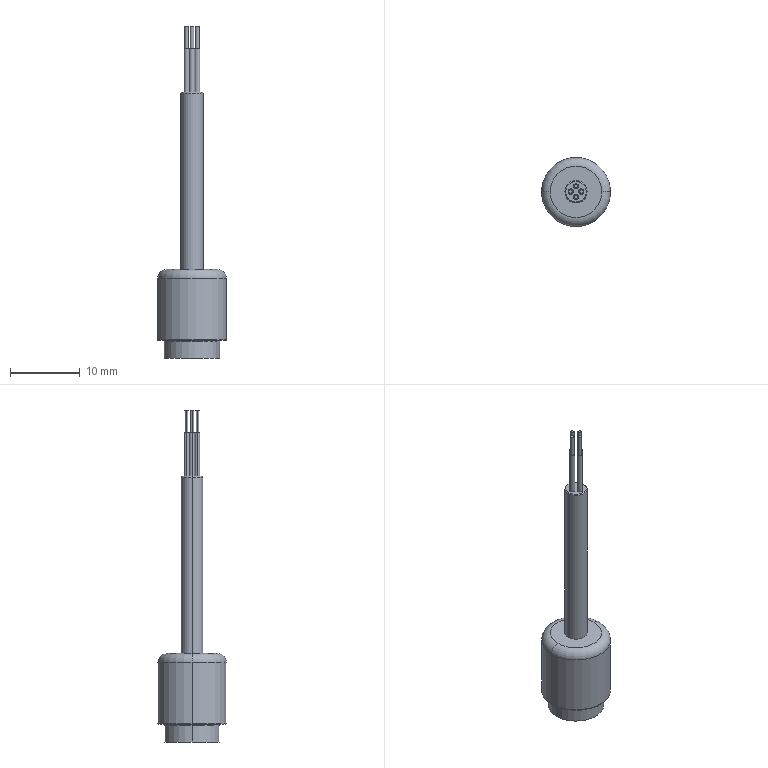Part | STEP file | CABLE | 1 solid | 42 faces | box 9.906 x 9.906 x 47.625 mm | volume 1114 mm3 | cylinder 22 | plane 12 | torus 8 | commonest cylinder face diameters 0.508 x8 0.762 x8 3.175 x2 7.938 x2 9.906 x2
STEP:
#1=CARTESIAN_POINT('',(-1.587,0.,35.433));
#2=VERTEX_POINT('',#1);
#3=CARTESIAN_POINT('',(1.587,0.,35.433));
#4=VERTEX_POINT('',#3);
#5=CARTESIAN_POINT('',(0.,0.,35.433));
#6=DIRECTION('',(0.,0.,-1.));
#7=DIRECTION('',(1.,0.,0.));
#8=AXIS2_PLACEMENT_3D('',#5,#6,#7);
#9=CIRCLE('',#8,1.587);
#10=EDGE_CURVE('',#2,#4,#9,.T.);
#11=ORIENTED_EDGE('',*,*,#10,.F.);
#12=CARTESIAN_POINT('',(-1.46,0.,35.56));
#13=VERTEX_POINT('',#12);
#14=CARTESIAN_POINT('',(-1.46,0.,35.433));
#15=DIRECTION('',(0.,1.,0.));
#16=DIRECTION('',(-1.,0.,0.));
#17=AXIS2_PLACEMENT_3D('',#14,#15,#16);
#18=CIRCLE('',#17,0.127);
#19=EDGE_CURVE('',#2,#13,#18,.T.);
#20=ORIENTED_EDGE('',*,*,#19,.T.);
#21=CARTESIAN_POINT('',(1.46,0.,35.56));
#22=VERTEX_POINT('',#21);
#23=CARTESIAN_POINT('',(0.,0.,35.56));
#24=DIRECTION('',(0.,0.,1.));
#25=DIRECTION('',(1.,0.,0.));
#26=AXIS2_PLACEMENT_3D('',#23,#24,#25);
#27=CIRCLE('',#26,1.46);
#28=EDGE_CURVE('',#22,#13,#27,.T.);
#29=ORIENTED_EDGE('',*,*,#28,.F.);
#30=CARTESIAN_POINT('',(1.46,0.,35.433));
#31=DIRECTION('',(0.,-1.,0.));
#32=DIRECTION('',(0.,0.,-1.));
#33=AXIS2_PLACEMENT_3D('',#30,#31,#32);
#34=CIRCLE('',#33,0.127);
#35=EDGE_CURVE('',#4,#22,#34,.T.);
#36=ORIENTED_EDGE('',*,*,#35,.F.);
#37=EDGE_LOOP('',(#11,#20,#29,#36));
#38=FACE_OUTER_BOUND('',#37,.T.);
#39=CARTESIAN_POINT('',(0.,0.,35.433));
#40=DIRECTION('',(0.,0.,1.));
#41=DIRECTION('',(1.,0.,0.));
#42=AXIS2_PLACEMENT_3D('',#39,#40,#41);
#43=TOROIDAL_SURFACE('',#42,1.46,0.127);
#44=ADVANCED_FACE('',(#38),#43,.T.);
#45=CARTESIAN_POINT('',(-0.508,0.,45.085));
#46=VERTEX_POINT('',#45);
#47=CARTESIAN_POINT('',(-1.016,0.,45.085));
#48=VERTEX_POINT('',#47);
#49=CARTESIAN_POINT('',(-0.762,0.,45.085));
#50=DIRECTION('',(0.,0.,1.));
#51=DIRECTION('',(1.,0.,0.));
#52=AXIS2_PLACEMENT_3D('',#49,#50,#51);
#53=CIRCLE('',#52,0.254);
#54=EDGE_CURVE('',#46,#48,#53,.T.);
#55=ORIENTED_EDGE('',*,*,#54,.F.);
#56=CARTESIAN_POINT('',(-0.508,0.,41.91));
#57=VERTEX_POINT('',#56);
#58=CARTESIAN_POINT('',(-0.508,0.,45.085));
#59=DIRECTION('',(0.,0.,-1.));
#60=VECTOR('',#59,1000.);
#61=LINE('',#58,#60);
#62=EDGE_CURVE('',#46,#57,#61,.T.);
#63=ORIENTED_EDGE('',*,*,#62,.T.);
#64=CARTESIAN_POINT('',(-1.016,0.,41.91));
#65=VERTEX_POINT('',#64);
#66=CARTESIAN_POINT('',(-0.762,0.,41.91));
#67=DIRECTION('',(0.,0.,-1.));
#68=DIRECTION('',(1.,0.,0.));
#69=AXIS2_PLACEMENT_3D('',#66,#67,#68);
#70=CIRCLE('',#69,0.254);
#71=EDGE_CURVE('',#65,#57,#70,.T.);
#72=ORIENTED_EDGE('',*,*,#71,.F.);
#73=CARTESIAN_POINT('',(-1.016,0.,45.085));
#74=DIRECTION('',(0.,0.,-1.));
#75=VECTOR('',#74,1000.);
#76=LINE('',#73,#75);
#77=EDGE_CURVE('',#48,#65,#76,.T.);
#78=ORIENTED_EDGE('',*,*,#77,.F.);
#79=EDGE_LOOP('',(#55,#63,#72,#78));
#80=FACE_OUTER_BOUND('',#79,.T.);
#81=CARTESIAN_POINT('',(-0.762,0.,45.085));
#82=DIRECTION('',(0.,0.,-1.));
#83=DIRECTION('',(-1.,0.,0.));
#84=AXIS2_PLACEMENT_3D('',#81,#82,#83);
#85=CYLINDRICAL_SURFACE('',#84,0.254);
#86=ADVANCED_FACE('',(#80),#85,.T.);
#87=CARTESIAN_POINT('',(-0.381,0.,41.91));
#88=VERTEX_POINT('',#87);
#89=CARTESIAN_POINT('',(-1.143,0.,41.91));
#90=VERTEX_POINT('',#89);
#91=CARTESIAN_POINT('',(-0.762,0.,41.91));
#92=DIRECTION('',(0.,0.,1.));
#93=DIRECTION('',(1.,0.,0.));
#94=AXIS2_PLACEMENT_3D('',#91,#92,#93);
#95=CIRCLE('',#94,0.381);
#96=EDGE_CURVE('',#88,#90,#95,.T.);
#97=ORIENTED_EDGE('',*,*,#96,.F.);
#98=CARTESIAN_POINT('',(-0.381,0.,35.56));
#99=VERTEX_POINT('',#98);
#100=CARTESIAN_POINT('',(-0.381,0.,41.91));
#101=DIRECTION('',(0.,0.,-1.));
#102=VECTOR('',#101,1000.);
#103=LINE('',#100,#102);
#104=EDGE_CURVE('',#88,#99,#103,.T.);
#105=ORIENTED_EDGE('',*,*,#104,.T.);
#106=CARTESIAN_POINT('',(-1.143,0.,35.56));
#107=VERTEX_POINT('',#106);
#108=CARTESIAN_POINT('',(-0.762,0.,35.56));
#109=DIRECTION('',(0.,0.,1.));
#110=DIRECTION('',(1.,0.,0.));
#111=AXIS2_PLACEMENT_3D('',#108,#109,#110);
#112=CIRCLE('',#111,0.381);
#113=EDGE_CURVE('',#99,#107,#112,.T.);
#114=ORIENTED_EDGE('',*,*,#113,.T.);
#115=CARTESIAN_POINT('',(-1.143,0.,41.91));
#116=DIRECTION('',(0.,0.,-1.));
#117=VECTOR('',#116,1000.);
#118=LINE('',#115,#117);
#119=EDGE_CURVE('',#90,#107,#118,.T.);
#120=ORIENTED_EDGE('',*,*,#119,.F.);
#121=EDGE_LOOP('',(#97,#105,#114,#120));
#122=FACE_OUTER_BOUND('',#121,.T.);
#123=CARTESIAN_POINT('',(-0.762,0.,41.91));
#124=DIRECTION('',(0.,0.,-1.));
#125=DIRECTION('',(-1.,0.,0.));
#126=AXIS2_PLACEMENT_3D('',#123,#124,#125);
#127=CYLINDRICAL_SURFACE('',#126,0.381);
#128=ADVANCED_FACE('',(#122),#127,.T.);
#129=CARTESIAN_POINT('',(0.254,0.762,45.085));
#130=VERTEX_POINT('',#129);
#131=CARTESIAN_POINT('',(-0.254,0.762,45.085));
#132=VERTEX_POINT('',#131);
#133=CARTESIAN_POINT('',(0.,0.762,45.085));
#134=DIRECTION('',(0.,0.,1.));
#135=DIRECTION('',(1.,0.,0.));
#136=AXIS2_PLACEMENT_3D('',#133,#134,#135);
#137=CIRCLE('',#136,0.254);
#138=EDGE_CURVE('',#130,#132,#137,.T.);
#139=ORIENTED_EDGE('',*,*,#138,.F.);
#140=CARTESIAN_POINT('',(0.254,0.762,41.91));
#141=VERTEX_POINT('',#140);
#142=CARTESIAN_POINT('',(0.254,0.762,45.085));
#143=DIRECTION('',(0.,0.,-1.));
#144=VECTOR('',#143,1000.);
#145=LINE('',#142,#144);
#146=EDGE_CURVE('',#130,#141,#145,.T.);
#147=ORIENTED_EDGE('',*,*,#146,.T.);
#148=CARTESIAN_POINT('',(-0.254,0.762,41.91));
#149=VERTEX_POINT('',#148);
#150=CARTESIAN_POINT('',(0.,0.762,41.91));
#151=DIRECTION('',(0.,0.,-1.));
#152=DIRECTION('',(1.,0.,0.));
#153=AXIS2_PLACEMENT_3D('',#150,#151,#152);
#154=CIRCLE('',#153,0.254);
#155=EDGE_CURVE('',#149,#141,#154,.T.);
#156=ORIENTED_EDGE('',*,*,#155,.F.);
#157=CARTESIAN_POINT('',(-0.254,0.762,45.085));
#158=DIRECTION('',(0.,0.,-1.));
#159=VECTOR('',#158,1000.);
#160=LINE('',#157,#159);
#161=EDGE_CURVE('',#132,#149,#160,.T.);
#162=ORIENTED_EDGE('',*,*,#161,.F.);
#163=EDGE_LOOP('',(#139,#147,#156,#162));
#164=FACE_OUTER_BOUND('',#163,.T.);
#165=CARTESIAN_POINT('',(0.,0.762,45.085));
#166=DIRECTION('',(0.,0.,-1.));
#167=DIRECTION('',(-1.,0.,0.));
#168=AXIS2_PLACEMENT_3D('',#165,#166,#167);
#169=CYLINDRICAL_SURFACE('',#168,0.254);
#170=ADVANCED_FACE('',(#164),#169,.T.);
#171=CARTESIAN_POINT('',(0.381,0.762,41.91));
#172=VERTEX_POINT('',#171);
#173=CARTESIAN_POINT('',(-0.381,0.762,41.91));
#174=VERTEX_POINT('',#173);
#175=CARTESIAN_POINT('',(0.,0.762,41.91));
#176=DIRECTION('',(0.,0.,1.));
#177=DIRECTION('',(1.,0.,0.));
#178=AXIS2_PLACEMENT_3D('',#175,#176,#177);
#179=CIRCLE('',#178,0.381);
#180=EDGE_CURVE('',#172,#174,#179,.T.);
#181=ORIENTED_EDGE('',*,*,#180,.F.);
#182=CARTESIAN_POINT('',(0.381,0.762,35.56));
#183=VERTEX_POINT('',#182);
#184=CARTESIAN_POINT('',(0.381,0.762,41.91));
#185=DIRECTION('',(0.,0.,-1.));
#186=VECTOR('',#185,1000.);
#187=LINE('',#184,#186);
#188=EDGE_CURVE('',#172,#183,#187,.T.);
#189=ORIENTED_EDGE('',*,*,#188,.T.);
#190=CARTESIAN_POINT('',(-0.381,0.762,35.56));
#191=VERTEX_POINT('',#190);
#192=CARTESIAN_POINT('',(0.,0.762,35.56));
#193=DIRECTION('',(0.,0.,1.));
#194=DIRECTION('',(1.,0.,0.));
#195=AXIS2_PLACEMENT_3D('',#192,#193,#194);
#196=CIRCLE('',#195,0.381);
#197=EDGE_CURVE('',#183,#191,#196,.T.);
#198=ORIENTED_EDGE('',*,*,#197,.T.);
#199=CARTESIAN_POINT('',(-0.381,0.762,41.91));
#200=DIRECTION('',(0.,0.,-1.));
#201=VECTOR('',#200,1000.);
#202=LINE('',#199,#201);
#203=EDGE_CURVE('',#174,#191,#202,.T.);
#204=ORIENTED_EDGE('',*,*,#203,.F.);
#205=EDGE_LOOP('',(#181,#189,#198,#204));
#206=FACE_OUTER_BOUND('',#205,.T.);
#207=CARTESIAN_POINT('',(0.,0.762,41.91));
#208=DIRECTION('',(0.,0.,-1.));
#209=DIRECTION('',(-1.,0.,0.));
#210=AXIS2_PLACEMENT_3D('',#207,#208,#209);
#211=CYLINDRICAL_SURFACE('',#210,0.381);
#212=ADVANCED_FACE('',(#206),#211,.T.);
#213=CARTESIAN_POINT('',(1.016,0.,45.085));
#214=VERTEX_POINT('',#213);
#215=CARTESIAN_POINT('',(0.508,0.,45.085));
#216=VERTEX_POINT('',#215);
#217=CARTESIAN_POINT('',(0.762,0.,45.085));
#218=DIRECTION('',(0.,0.,1.));
#219=DIRECTION('',(1.,0.,0.));
#220=AXIS2_PLACEMENT_3D('',#217,#218,#219);
#221=CIRCLE('',#220,0.254);
#222=EDGE_CURVE('',#214,#216,#221,.T.);
#223=ORIENTED_EDGE('',*,*,#222,.F.);
#224=CARTESIAN_POINT('',(1.016,0.,41.91));
#225=VERTEX_POINT('',#224);
#226=CARTESIAN_POINT('',(1.016,0.,45.085));
#227=DIRECTION('',(0.,0.,-1.));
#228=VECTOR('',#227,1000.);
#229=LINE('',#226,#228);
#230=EDGE_CURVE('',#214,#225,#229,.T.);
#231=ORIENTED_EDGE('',*,*,#230,.T.);
#232=CARTESIAN_POINT('',(0.508,0.,41.91));
#233=VERTEX_POINT('',#232);
#234=CARTESIAN_POINT('',(0.762,0.,41.91));
#235=DIRECTION('',(0.,0.,-1.));
#236=DIRECTION('',(1.,0.,0.));
#237=AXIS2_PLACEMENT_3D('',#234,#235,#236);
#238=CIRCLE('',#237,0.254);
#239=EDGE_CURVE('',#233,#225,#238,.T.);
#240=ORIENTED_EDGE('',*,*,#239,.F.);
#241=CARTESIAN_POINT('',(0.508,0.,45.085));
#242=DIRECTION('',(0.,0.,-1.));
#243=VECTOR('',#242,1000.);
#244=LINE('',#241,#243);
#245=EDGE_CURVE('',#216,#233,#244,.T.);
#246=ORIENTED_EDGE('',*,*,#245,.F.);
#247=EDGE_LOOP('',(#223,#231,#240,#246));
#248=FACE_OUTER_BOUND('',#247,.T.);
#249=CARTESIAN_POINT('',(0.762,0.,45.085));
#250=DIRECTION('',(0.,0.,-1.));
#251=DIRECTION('',(-1.,0.,0.));
#252=AXIS2_PLACEMENT_3D('',#249,#250,#251);
#253=CYLINDRICAL_SURFACE('',#252,0.254);
#254=ADVANCED_FACE('',(#248),#253,.T.);
#255=CARTESIAN_POINT('',(1.143,0.,41.91));
#256=VERTEX_POINT('',#255);
#257=CARTESIAN_POINT('',(0.381,0.,41.91));
#258=VERTEX_POINT('',#257);
#259=CARTESIAN_POINT('',(0.762,0.,41.91));
#260=DIRECTION('',(0.,0.,1.));
#261=DIRECTION('',(1.,0.,0.));
#262=AXIS2_PLACEMENT_3D('',#259,#260,#261);
#263=CIRCLE('',#262,0.381);
#264=EDGE_CURVE('',#256,#258,#263,.T.);
#265=ORIENTED_EDGE('',*,*,#264,.F.);
#266=CARTESIAN_POINT('',(1.143,0.,35.56));
#267=VERTEX_POINT('',#266);
#268=CARTESIAN_POINT('',(1.143,0.,41.91));
#269=DIRECTION('',(0.,0.,-1.));
#270=VECTOR('',#269,1000.);
#271=LINE('',#268,#270);
#272=EDGE_CURVE('',#256,#267,#271,.T.);
#273=ORIENTED_EDGE('',*,*,#272,.T.);
#274=CARTESIAN_POINT('',(0.381,0.,35.56));
#275=VERTEX_POINT('',#274);
#276=CARTESIAN_POINT('',(0.762,0.,35.56));
#277=DIRECTION('',(0.,0.,1.));
#278=DIRECTION('',(1.,0.,0.));
#279=AXIS2_PLACEMENT_3D('',#276,#277,#278);
#280=CIRCLE('',#279,0.381);
#281=EDGE_CURVE('',#267,#275,#280,.T.);
#282=ORIENTED_EDGE('',*,*,#281,.T.);
#283=CARTESIAN_POINT('',(0.381,0.,41.91));
#284=DIRECTION('',(0.,0.,-1.));
#285=VECTOR('',#284,1000.);
#286=LINE('',#283,#285);
#287=EDGE_CURVE('',#258,#275,#286,.T.);
#288=ORIENTED_EDGE('',*,*,#287,.F.);
#289=EDGE_LOOP('',(#265,#273,#282,#288));
#290=FACE_OUTER_BOUND('',#289,.T.);
#291=CARTESIAN_POINT('',(0.762,0.,41.91));
#292=DIRECTION('',(0.,0.,-1.));
#293=DIRECTION('',(-1.,0.,0.));
#294=AXIS2_PLACEMENT_3D('',#291,#292,#293);
#295=CYLINDRICAL_SURFACE('',#294,0.381);
#296=ADVANCED_FACE('',(#290),#295,.T.);
#297=CARTESIAN_POINT('',(0.254,-0.762,45.085));
#298=VERTEX_POINT('',#297);
#299=CARTESIAN_POINT('',(-0.254,-0.762,45.085));
#300=VERTEX_POINT('',#299);
#301=CARTESIAN_POINT('',(0.,-0.762,45.085));
#302=DIRECTION('',(0.,0.,1.));
#303=DIRECTION('',(1.,0.,0.));
#304=AXIS2_PLACEMENT_3D('',#301,#302,#303);
#305=CIRCLE('',#304,0.254);
#306=EDGE_CURVE('',#298,#300,#305,.T.);
#307=ORIENTED_EDGE('',*,*,#306,.F.);
#308=CARTESIAN_POINT('',(0.254,-0.762,41.91));
#309=VERTEX_POINT('',#308);
#310=CARTESIAN_POINT('',(0.254,-0.762,45.085));
#311=DIRECTION('',(0.,0.,-1.));
#312=VECTOR('',#311,1000.);
#313=LINE('',#310,#312);
#314=EDGE_CURVE('',#298,#309,#313,.T.);
#315=ORIENTED_EDGE('',*,*,#314,.T.);
#316=CARTESIAN_POINT('',(-0.254,-0.762,41.91));
#317=VERTEX_POINT('',#316);
#318=CARTESIAN_POINT('',(0.,-0.762,41.91));
#319=DIRECTION('',(0.,0.,-1.));
#320=DIRECTION('',(1.,0.,0.));
#321=AXIS2_PLACEMENT_3D('',#318,#319,#320);
#322=CIRCLE('',#321,0.254);
#323=EDGE_CURVE('',#317,#309,#322,.T.);
#324=ORIENTED_EDGE('',*,*,#323,.F.);
#325=CARTESIAN_POINT('',(-0.254,-0.762,45.085));
#326=DIRECTION('',(0.,0.,-1.));
#327=VECTOR('',#326,1000.);
#328=LINE('',#325,#327);
#329=EDGE_CURVE('',#300,#317,#328,.T.);
#330=ORIENTED_EDGE('',*,*,#329,.F.);
#331=EDGE_LOOP('',(#307,#315,#324,#330));
#332=FACE_OUTER_BOUND('',#331,.T.);
#333=CARTESIAN_POINT('',(0.,-0.762,45.085));
#334=DIRECTION('',(0.,0.,-1.));
#335=DIRECTION('',(-1.,0.,0.));
#336=AXIS2_PLACEMENT_3D('',#333,#334,#335);
#337=CYLINDRICAL_SURFACE('',#336,0.254);
#338=ADVANCED_FACE('',(#332),#337,.T.);
#339=CARTESIAN_POINT('',(0.381,-0.762,41.91));
#340=VERTEX_POINT('',#339);
#341=CARTESIAN_POINT('',(-0.381,-0.762,41.91));
#342=VERTEX_POINT('',#341);
#343=CARTESIAN_POINT('',(0.,-0.762,41.91));
#344=DIRECTION('',(0.,0.,1.));
#345=DIRECTION('',(1.,0.,0.));
#346=AXIS2_PLACEMENT_3D('',#343,#344,#345);
#347=CIRCLE('',#346,0.381);
#348=EDGE_CURVE('',#340,#342,#347,.T.);
#349=ORIENTED_EDGE('',*,*,#348,.F.);
#350=CARTESIAN_POINT('',(0.381,-0.762,35.56));
#351=VERTEX_POINT('',#350);
#352=CARTESIAN_POINT('',(0.381,-0.762,41.91));
#353=DIRECTION('',(0.,0.,-1.));
#354=VECTOR('',#353,1000.);
#355=LINE('',#352,#354);
#356=EDGE_CURVE('',#340,#351,#355,.T.);
#357=ORIENTED_EDGE('',*,*,#356,.T.);
#358=CARTESIAN_POINT('',(-0.381,-0.762,35.56));
#359=VERTEX_POINT('',#358);
#360=CARTESIAN_POINT('',(0.,-0.762,35.56));
#361=DIRECTION('',(0.,0.,1.));
#362=DIRECTION('',(1.,0.,0.));
#363=AXIS2_PLACEMENT_3D('',#360,#361,#362);
#364=CIRCLE('',#363,0.381);
#365=EDGE_CURVE('',#351,#359,#364,.T.);
#366=ORIENTED_EDGE('',*,*,#365,.T.);
#367=CARTESIAN_POINT('',(-0.381,-0.762,41.91));
#368=DIRECTION('',(0.,0.,-1.));
#369=VECTOR('',#368,1000.);
#370=LINE('',#367,#369);
#371=EDGE_CURVE('',#342,#359,#370,.T.);
#372=ORIENTED_EDGE('',*,*,#371,.F.);
#373=EDGE_LOOP('',(#349,#357,#366,#372));
#374=FACE_OUTER_BOUND('',#373,.T.);
#375=CARTESIAN_POINT('',(0.,-0.762,41.91));
#376=DIRECTION('',(0.,0.,-1.));
#377=DIRECTION('',(-1.,0.,0.));
#378=AXIS2_PLACEMENT_3D('',#375,#376,#377);
#379=CYLINDRICAL_SURFACE('',#378,0.381);
#380=ADVANCED_FACE('',(#374),#379,.T.);
#381=CARTESIAN_POINT('',(-4.953,0.,8.89));
#382=VERTEX_POINT('',#381);
#383=CARTESIAN_POINT('',(4.953,0.,8.89));
#384=VERTEX_POINT('',#383);
#385=CARTESIAN_POINT('',(0.,0.,8.89));
#386=DIRECTION('',(0.,0.,-1.));
#387=DIRECTION('',(1.,0.,0.));
#388=AXIS2_PLACEMENT_3D('',#385,#386,#387);
#389=CIRCLE('',#388,4.953);
#390=EDGE_CURVE('',#382,#384,#389,.T.);
#391=ORIENTED_EDGE('',*,*,#390,.F.);
#392=CARTESIAN_POINT('',(-3.683,0.,10.16));
#393=VERTEX_POINT('',#392);
#394=CARTESIAN_POINT('',(-3.683,0.,8.89));
#395=DIRECTION('',(0.,1.,0.));
#396=DIRECTION('',(-1.,0.,0.));
#397=AXIS2_PLACEMENT_3D('',#394,#395,#396);
#398=CIRCLE('',#397,1.27);
#399=EDGE_CURVE('',#382,#393,#398,.T.);
#400=ORIENTED_EDGE('',*,*,#399,.T.);
#401=CARTESIAN_POINT('',(3.683,0.,10.16));
#402=VERTEX_POINT('',#401);
#403=CARTESIAN_POINT('',(0.,0.,10.16));
#404=DIRECTION('',(0.,0.,1.));
#405=DIRECTION('',(1.,0.,0.));
#406=AXIS2_PLACEMENT_3D('',#403,#404,#405);
#407=CIRCLE('',#406,3.683);
#408=EDGE_CURVE('',#402,#393,#407,.T.);
#409=ORIENTED_EDGE('',*,*,#408,.F.);
#410=CARTESIAN_POINT('',(3.683,0.,8.89));
#411=DIRECTION('',(0.,-1.,0.));
#412=DIRECTION('',(0.,0.,-1.));
#413=AXIS2_PLACEMENT_3D('',#410,#411,#412);
#414=CIRCLE('',#413,1.27);
#415=EDGE_CURVE('',#384,#402,#414,.T.);
#416=ORIENTED_EDGE('',*,*,#415,.F.);
#417=EDGE_LOOP('',(#391,#400,#409,#416));
#418=FACE_OUTER_BOUND('',#417,.T.);
#419=CARTESIAN_POINT('',(0.,0.,8.89));
#420=DIRECTION('',(0.,0.,1.));
#421=DIRECTION('',(1.,0.,0.));
#422=AXIS2_PLACEMENT_3D('',#419,#420,#421);
#423=TOROIDAL_SURFACE('',#422,3.683,1.27);
#424=ADVANCED_FACE('',(#418),#423,.T.);
#425=CARTESIAN_POINT('',(-4.826,0.,0.));
#426=VERTEX_POINT('',#425);
#427=CARTESIAN_POINT('',(4.826,0.,0.));
#428=VERTEX_POINT('',#427);
#429=CARTESIAN_POINT('',(0.,0.,0.));
#430=DIRECTION('',(0.,0.,-1.));
#431=DIRECTION('',(1.,0.,0.));
#432=AXIS2_PLACEMENT_3D('',#429,#430,#431);
#433=CIRCLE('',#432,4.826);
#434=EDGE_CURVE('',#426,#428,#433,.T.);
#435=ORIENTED_EDGE('',*,*,#434,.F.);
#436=CARTESIAN_POINT('',(-4.953,0.,0.127));
#437=VERTEX_POINT('',#436);
#438=CARTESIAN_POINT('',(-4.826,0.,0.127));
#439=DIRECTION('',(0.,1.,0.));
#440=DIRECTION('',(-1.,0.,0.));
#441=AXIS2_PLACEMENT_3D('',#438,#439,#440);
#442=CIRCLE('',#441,0.127);
#443=EDGE_CURVE('',#426,#437,#442,.T.);
#444=ORIENTED_EDGE('',*,*,#443,.T.);
#445=CARTESIAN_POINT('',(4.953,0.,0.127));
#446=VERTEX_POINT('',#445);
#447=CARTESIAN_POINT('',(0.,0.,0.127));
#448=DIRECTION('',(0.,0.,1.));
#449=DIRECTION('',(1.,0.,0.));
#450=AXIS2_PLACEMENT_3D('',#447,#448,#449);
#451=CIRCLE('',#450,4.953);
#452=EDGE_CURVE('',#446,#437,#451,.T.);
#453=ORIENTED_EDGE('',*,*,#452,.F.);
#454=CARTESIAN_POINT('',(4.826,0.,0.127));
#455=DIRECTION('',(0.,-1.,0.));
#456=DIRECTION('',(0.,0.,-1.));
#457=AXIS2_PLACEMENT_3D('',#454,#455,#456);
#458=CIRCLE('',#457,0.127);
#459=EDGE_CURVE('',#428,#446,#458,.T.);
#460=ORIENTED_EDGE('',*,*,#459,.F.);
#461=EDGE_LOOP('',(#435,#444,#453,#460));
#462=FACE_OUTER_BOUND('',#461,.T.);
#463=CARTESIAN_POINT('',(0.,0.,0.127));
#464=DIRECTION('',(0.,0.,1.));
#465=DIRECTION('',(1.,0.,0.));
#466=AXIS2_PLACEMENT_3D('',#463,#464,#465);
#467=TOROIDAL_SURFACE('',#466,4.826,0.127);
#468=ADVANCED_FACE('',(#462),#467,.T.);
#469=CARTESIAN_POINT('',(-4.096,0.,0.));
#470=VERTEX_POINT('',#469);
#471=CARTESIAN_POINT('',(4.096,0.,0.));
#472=VERTEX_POINT('',#471);
#473=CARTESIAN_POINT('',(0.,0.,0.));
#474=DIRECTION('',(0.,0.,1.));
#475=DIRECTION('',(1.,0.,0.));
#476=AXIS2_PLACEMENT_3D('',#473,#474,#475);
#477=CIRCLE('',#476,4.096);
#478=EDGE_CURVE('',#470,#472,#477,.T.);
#479=ORIENTED_EDGE('',*,*,#478,.F.);
#480=CARTESIAN_POINT('',(-3.969,0.,-0.127));
#481=VERTEX_POINT('',#480);
#482=CARTESIAN_POINT('',(-4.096,0.,-0.127));
#483=DIRECTION('',(0.,1.,0.));
#484=DIRECTION('',(-1.,0.,0.));
#485=AXIS2_PLACEMENT_3D('',#482,#483,#484);
#486=CIRCLE('',#485,0.127);
#487=EDGE_CURVE('',#470,#481,#486,.T.);
#488=ORIENTED_EDGE('',*,*,#487,.T.);
#489=CARTESIAN_POINT('',(3.969,0.,-0.127));
#490=VERTEX_POINT('',#489);
#491=CARTESIAN_POINT('',(0.,0.,-0.127));
#492=DIRECTION('',(0.,0.,-1.));
#493=DIRECTION('',(1.,0.,0.));
#494=AXIS2_PLACEMENT_3D('',#491,#492,#493);
#495=CIRCLE('',#494,3.969);
#496=EDGE_CURVE('',#490,#481,#495,.T.);
#497=ORIENTED_EDGE('',*,*,#496,.F.);
#498=CARTESIAN_POINT('',(4.096,0.,-0.127));
#499=DIRECTION('',(0.,-1.,0.));
#500=DIRECTION('',(0.,0.,-1.));
#501=AXIS2_PLACEMENT_3D('',#498,#499,#500);
#502=CIRCLE('',#501,0.127);
#503=EDGE_CURVE('',#472,#490,#502,.T.);
#504=ORIENTED_EDGE('',*,*,#503,.F.);
#505=EDGE_LOOP('',(#479,#488,#497,#504));
#506=FACE_OUTER_BOUND('',#505,.T.);
#507=CARTESIAN_POINT('',(0.,0.,-0.127));
#508=DIRECTION('',(0.,0.,1.));
#509=DIRECTION('',(1.,0.,0.));
#510=AXIS2_PLACEMENT_3D('',#507,#508,#509);
#511=TOROIDAL_SURFACE('',#510,4.096,0.127);
#512=ADVANCED_FACE('',(#506),#511,.F.);
#513=ORIENTED_EDGE('',*,*,#10,.T.);
#514=CARTESIAN_POINT('',(1.587,0.,10.16));
#515=VERTEX_POINT('',#514);
#516=CARTESIAN_POINT('',(1.587,0.,35.56));
#517=DIRECTION('',(0.,0.,-1.));
#518=VECTOR('',#517,1000.);
#519=LINE('',#516,#518);
#520=EDGE_CURVE('',#4,#515,#519,.T.);
#521=ORIENTED_EDGE('',*,*,#520,.T.);
#522=CARTESIAN_POINT('',(-1.587,0.,10.16));
#523=VERTEX_POINT('',#522);
#524=CARTESIAN_POINT('',(0.,0.,10.16));
#525=DIRECTION('',(0.,0.,1.));
#526=DIRECTION('',(1.,0.,0.));
#527=AXIS2_PLACEMENT_3D('',#524,#525,#526);
#528=CIRCLE('',#527,1.587);
#529=EDGE_CURVE('',#515,#523,#528,.T.);
#530=ORIENTED_EDGE('',*,*,#529,.T.);
#531=CARTESIAN_POINT('',(-1.587,0.,35.56));
#532=DIRECTION('',(0.,0.,-1.));
#533=VECTOR('',#532,1000.);
#534=LINE('',#531,#533);
#535=EDGE_CURVE('',#2,#523,#534,.T.);
#536=ORIENTED_EDGE('',*,*,#535,.F.);
#537=EDGE_LOOP('',(#513,#521,#530,#536));
#538=FACE_OUTER_BOUND('',#537,.T.);
#539=CARTESIAN_POINT('',(0.,0.,35.56));
#540=DIRECTION('',(0.,0.,-1.));
#541=DIRECTION('',(-1.,0.,0.));
#542=AXIS2_PLACEMENT_3D('',#539,#540,#541);
#543=CYLINDRICAL_SURFACE('',#542,1.587);
#544=ADVANCED_FACE('',(#538),#543,.T.);
#545=CARTESIAN_POINT('',(3.969,0.,-2.54));
#546=VERTEX_POINT('',#545);
#547=CARTESIAN_POINT('',(-3.969,0.,-2.54));
#548=VERTEX_POINT('',#547);
#549=CARTESIAN_POINT('',(0.,0.,-2.54));
#550=DIRECTION('',(0.,0.,1.));
#551=DIRECTION('',(1.,0.,0.));
#552=AXIS2_PLACEMENT_3D('',#549,#550,#551);
#553=CIRCLE('',#552,3.969);
#554=EDGE_CURVE('',#546,#548,#553,.T.);
#555=ORIENTED_EDGE('',*,*,#554,.T.);
#556=CARTESIAN_POINT('',(-3.969,0.,-2.54));
#557=DIRECTION('',(0.,0.,1.));
#558=VECTOR('',#557,1000.);
#559=LINE('',#556,#558);
#560=EDGE_CURVE('',#548,#481,#559,.T.);
#561=ORIENTED_EDGE('',*,*,#560,.T.);
#562=CARTESIAN_POINT('',(0.,0.,-0.127));
#563=DIRECTION('',(0.,0.,-1.));
#564=DIRECTION('',(1.,0.,0.));
#565=AXIS2_PLACEMENT_3D('',#562,#563,#564);
#566=CIRCLE('',#565,3.969);
#567=EDGE_CURVE('',#481,#490,#566,.T.);
#568=ORIENTED_EDGE('',*,*,#567,.T.);
#569=CARTESIAN_POINT('',(3.969,0.,-2.54));
#570=DIRECTION('',(0.,0.,1.));
#571=VECTOR('',#570,1000.);
#572=LINE('',#569,#571);
#573=EDGE_CURVE('',#546,#490,#572,.T.);
#574=ORIENTED_EDGE('',*,*,#573,.F.);
#575=EDGE_LOOP('',(#555,#561,#568,#574));
#576=FACE_OUTER_BOUND('',#575,.T.);
#577=CARTESIAN_POINT('',(0.,0.,-2.54));
#578=DIRECTION('',(0.,0.,1.));
#579=DIRECTION('',(1.,0.,0.));
#580=AXIS2_PLACEMENT_3D('',#577,#578,#579);
#581=CYLINDRICAL_SURFACE('',#580,3.969);
#582=ADVANCED_FACE('',(#576),#581,.T.);
#583=ORIENTED_EDGE('',*,*,#390,.T.);
#584=CARTESIAN_POINT('',(4.953,0.,10.16));
#585=DIRECTION('',(0.,0.,-1.));
#586=VECTOR('',#585,1000.);
#587=LINE('',#584,#586);
#588=EDGE_CURVE('',#384,#446,#587,.T.);
#589=ORIENTED_EDGE('',*,*,#588,.T.);
#590=ORIENTED_EDGE('',*,*,#452,.T.);
#591=CARTESIAN_POINT('',(-4.953,0.,10.16));
#592=DIRECTION('',(0.,0.,-1.));
#593=VECTOR('',#592,1000.);
#594=LINE('',#591,#593);
#595=EDGE_CURVE('',#382,#437,#594,.T.);
#596=ORIENTED_EDGE('',*,*,#595,.F.);
#597=EDGE_LOOP('',(#583,#589,#590,#596));
#598=FACE_OUTER_BOUND('',#597,.T.);
#599=CARTESIAN_POINT('',(0.,0.,10.16));
#600=DIRECTION('',(0.,0.,-1.));
#601=DIRECTION('',(-1.,0.,0.));
#602=AXIS2_PLACEMENT_3D('',#599,#600,#601);
#603=CYLINDRICAL_SURFACE('',#602,4.953);
#604=ADVANCED_FACE('',(#598),#603,.T.);
#605=ORIENTED_EDGE('',*,*,#28,.T.);
#606=CARTESIAN_POINT('',(0.,0.,35.56));
#607=DIRECTION('',(0.,0.,1.));
#608=DIRECTION('',(1.,0.,0.));
#609=AXIS2_PLACEMENT_3D('',#606,#607,#608);
#610=CIRCLE('',#609,1.46);
#611=EDGE_CURVE('',#13,#22,#610,.T.);
#612=ORIENTED_EDGE('',*,*,#611,.T.);
#613=EDGE_LOOP('',(#605,#612));
#614=FACE_OUTER_BOUND('',#613,.T.);
#615=CARTESIAN_POINT('',(0.,0.762,35.56));
#616=DIRECTION('',(0.,0.,1.));
#617=DIRECTION('',(1.,0.,0.));
#618=AXIS2_PLACEMENT_3D('',#615,#616,#617);
#619=CIRCLE('',#618,0.381);
#620=EDGE_CURVE('',#191,#183,#619,.T.);
#621=ORIENTED_EDGE('',*,*,#620,.F.);
#622=ORIENTED_EDGE('',*,*,#197,.F.);
#623=EDGE_LOOP('',(#621,#622));
#624=FACE_BOUND('',#623,.T.);
#625=CARTESIAN_POINT('',(0.,-0.762,35.56));
#626=DIRECTION('',(0.,0.,1.));
#627=DIRECTION('',(1.,0.,0.));
#628=AXIS2_PLACEMENT_3D('',#625,#626,#627);
#629=CIRCLE('',#628,0.381);
#630=EDGE_CURVE('',#359,#351,#629,.T.);
#631=ORIENTED_EDGE('',*,*,#630,.F.);
#632=ORIENTED_EDGE('',*,*,#365,.F.);
#633=EDGE_LOOP('',(#631,#632));
#634=FACE_BOUND('',#633,.T.);
#635=CARTESIAN_POINT('',(0.762,0.,35.56));
#636=DIRECTION('',(0.,0.,1.));
#637=DIRECTION('',(1.,0.,0.));
#638=AXIS2_PLACEMENT_3D('',#635,#636,#637);
#639=CIRCLE('',#638,0.381);
#640=EDGE_CURVE('',#275,#267,#639,.T.);
#641=ORIENTED_EDGE('',*,*,#640,.F.);
#642=ORIENTED_EDGE('',*,*,#281,.F.);
#643=EDGE_LOOP('',(#641,#642));
#644=FACE_BOUND('',#643,.T.);
#645=CARTESIAN_POINT('',(-0.762,0.,35.56));
#646=DIRECTION('',(0.,0.,1.));
#647=DIRECTION('',(1.,0.,0.));
#648=AXIS2_PLACEMENT_3D('',#645,#646,#647);
#649=CIRCLE('',#648,0.381);
#650=EDGE_CURVE('',#107,#99,#649,.T.);
#651=ORIENTED_EDGE('',*,*,#650,.F.);
#652=ORIENTED_EDGE('',*,*,#113,.F.);
#653=EDGE_LOOP('',(#651,#652));
#654=FACE_BOUND('',#653,.T.);
#655=CARTESIAN_POINT('',(0.,0.,35.56));
#656=DIRECTION('',(0.,0.,1.));
#657=DIRECTION('',(1.,0.,0.));
#658=AXIS2_PLACEMENT_3D('',#655,#656,#657);
#659=PLANE('',#658);
#660=ADVANCED_FACE('',(#614,#624,#634,#644,#654),#659,.T.);
#661=ORIENTED_EDGE('',*,*,#408,.T.);
#662=CARTESIAN_POINT('',(0.,0.,10.16));
#663=DIRECTION('',(0.,0.,1.));
#664=DIRECTION('',(1.,0.,0.));
#665=AXIS2_PLACEMENT_3D('',#662,#663,#664);
#666=CIRCLE('',#665,3.683);
#667=EDGE_CURVE('',#393,#402,#666,.T.);
#668=ORIENTED_EDGE('',*,*,#667,.T.);
#669=EDGE_LOOP('',(#661,#668));
#670=FACE_OUTER_BOUND('',#669,.T.);
#671=CARTESIAN_POINT('',(0.,0.,10.16));
#672=DIRECTION('',(0.,0.,1.));
#673=DIRECTION('',(1.,0.,0.));
#674=AXIS2_PLACEMENT_3D('',#671,#672,#673);
#675=CIRCLE('',#674,1.587);
#676=EDGE_CURVE('',#523,#515,#675,.T.);
#677=ORIENTED_EDGE('',*,*,#676,.F.);
#678=ORIENTED_EDGE('',*,*,#529,.F.);
#679=EDGE_LOOP('',(#677,#678));
#680=FACE_BOUND('',#679,.T.);
#681=CARTESIAN_POINT('',(0.,0.,10.16));
#682=DIRECTION('',(0.,0.,1.));
#683=DIRECTION('',(1.,0.,0.));
#684=AXIS2_PLACEMENT_3D('',#681,#682,#683);
#685=PLANE('',#684);
#686=ADVANCED_FACE('',(#670,#680),#685,.T.);
#687=ORIENTED_EDGE('',*,*,#588,.F.);
#688=CARTESIAN_POINT('',(0.,0.,8.89));
#689=DIRECTION('',(0.,0.,-1.));
#690=DIRECTION('',(1.,0.,0.));
#691=AXIS2_PLACEMENT_3D('',#688,#689,#690);
#692=CIRCLE('',#691,4.953);
#693=EDGE_CURVE('',#384,#382,#692,.T.);
#694=ORIENTED_EDGE('',*,*,#693,.T.);
#695=ORIENTED_EDGE('',*,*,#595,.T.);
#696=CARTESIAN_POINT('',(0.,0.,0.127));
#697=DIRECTION('',(0.,0.,1.));
#698=DIRECTION('',(1.,0.,0.));
#699=AXIS2_PLACEMENT_3D('',#696,#697,#698);
#700=CIRCLE('',#699,4.953);
#701=EDGE_CURVE('',#437,#446,#700,.T.);
#702=ORIENTED_EDGE('',*,*,#701,.T.);
#703=EDGE_LOOP('',(#687,#694,#695,#702));
#704=FACE_OUTER_BOUND('',#703,.T.);
#705=CARTESIAN_POINT('',(0.,0.,10.16));
#706=DIRECTION('',(0.,0.,-1.));
#707=DIRECTION('',(-1.,0.,0.));
#708=AXIS2_PLACEMENT_3D('',#705,#706,#707);
#709=CYLINDRICAL_SURFACE('',#708,4.953);
#710=ADVANCED_FACE('',(#704),#709,.T.);
#711=CARTESIAN_POINT('',(0.,0.,0.));
#712=DIRECTION('',(0.,0.,1.));
#713=DIRECTION('',(1.,0.,0.));
#714=AXIS2_PLACEMENT_3D('',#711,#712,#713);
#715=CIRCLE('',#714,4.096);
#716=EDGE_CURVE('',#472,#470,#715,.T.);
#717=ORIENTED_EDGE('',*,*,#716,.T.);
#718=ORIENTED_EDGE('',*,*,#478,.T.);
#719=EDGE_LOOP('',(#717,#718));
#720=FACE_BOUND('',#719,.T.);
#721=CARTESIAN_POINT('',(0.,0.,0.));
#722=DIRECTION('',(0.,0.,-1.));
#723=DIRECTION('',(1.,0.,0.));
#724=AXIS2_PLACEMENT_3D('',#721,#722,#723);
#725=CIRCLE('',#724,4.826);
#726=EDGE_CURVE('',#428,#426,#725,.T.);
#727=ORIENTED_EDGE('',*,*,#726,.T.);
#728=ORIENTED_EDGE('',*,*,#434,.T.);
#729=EDGE_LOOP('',(#727,#728));
#730=FACE_OUTER_BOUND('',#729,.T.);
#731=CARTESIAN_POINT('',(0.,0.,0.));
#732=DIRECTION('',(0.,0.,1.));
#733=DIRECTION('',(1.,0.,0.));
#734=AXIS2_PLACEMENT_3D('',#731,#732,#733);
#735=PLANE('',#734);
#736=ADVANCED_FACE('',(#720,#730),#735,.F.);
#737=ORIENTED_EDGE('',*,*,#560,.F.);
#738=CARTESIAN_POINT('',(0.,0.,-2.54));
#739=DIRECTION('',(0.,0.,1.));
#740=DIRECTION('',(1.,0.,0.));
#741=AXIS2_PLACEMENT_3D('',#738,#739,#740);
#742=CIRCLE('',#741,3.969);
#743=EDGE_CURVE('',#548,#546,#742,.T.);
#744=ORIENTED_EDGE('',*,*,#743,.T.);
#745=ORIENTED_EDGE('',*,*,#573,.T.);
#746=ORIENTED_EDGE('',*,*,#496,.T.);
#747=EDGE_LOOP('',(#737,#744,#745,#746));
#748=FACE_OUTER_BOUND('',#747,.T.);
#749=CARTESIAN_POINT('',(0.,0.,-2.54));
#750=DIRECTION('',(0.,0.,1.));
#751=DIRECTION('',(1.,0.,0.));
#752=AXIS2_PLACEMENT_3D('',#749,#750,#751);
#753=CYLINDRICAL_SURFACE('',#752,3.969);
#754=ADVANCED_FACE('',(#748),#753,.T.);
#755=ORIENTED_EDGE('',*,*,#554,.F.);
#756=ORIENTED_EDGE('',*,*,#743,.F.);
#757=EDGE_LOOP('',(#755,#756));
#758=FACE_OUTER_BOUND('',#757,.T.);
#759=CARTESIAN_POINT('',(0.,0.,-2.54));
#760=DIRECTION('',(0.,0.,1.));
#761=DIRECTION('',(1.,0.,0.));
#762=AXIS2_PLACEMENT_3D('',#759,#760,#761);
#763=PLANE('',#762);
#764=ADVANCED_FACE('',(#758),#763,.F.);
#765=ORIENTED_EDGE('',*,*,#520,.F.);
#766=CARTESIAN_POINT('',(0.,0.,35.433));
#767=DIRECTION('',(0.,0.,-1.));
#768=DIRECTION('',(1.,0.,0.));
#769=AXIS2_PLACEMENT_3D('',#766,#767,#768);
#770=CIRCLE('',#769,1.587);
#771=EDGE_CURVE('',#4,#2,#770,.T.);
#772=ORIENTED_EDGE('',*,*,#771,.T.);
#773=ORIENTED_EDGE('',*,*,#535,.T.);
#774=ORIENTED_EDGE('',*,*,#676,.T.);
#775=EDGE_LOOP('',(#765,#772,#773,#774));
#776=FACE_OUTER_BOUND('',#775,.T.);
#777=CARTESIAN_POINT('',(0.,0.,35.56));
#778=DIRECTION('',(0.,0.,-1.));
#779=DIRECTION('',(-1.,0.,0.));
#780=AXIS2_PLACEMENT_3D('',#777,#778,#779);
#781=CYLINDRICAL_SURFACE('',#780,1.587);
#782=ADVANCED_FACE('',(#776),#781,.T.);
#783=ORIENTED_EDGE('',*,*,#487,.F.);
#784=ORIENTED_EDGE('',*,*,#716,.F.);
#785=ORIENTED_EDGE('',*,*,#503,.T.);
#786=ORIENTED_EDGE('',*,*,#567,.F.);
#787=EDGE_LOOP('',(#783,#784,#785,#786));
#788=FACE_OUTER_BOUND('',#787,.T.);
#789=CARTESIAN_POINT('',(0.,0.,-0.127));
#790=DIRECTION('',(0.,0.,1.));
#791=DIRECTION('',(1.,0.,0.));
#792=AXIS2_PLACEMENT_3D('',#789,#790,#791);
#793=TOROIDAL_SURFACE('',#792,4.096,0.127);
#794=ADVANCED_FACE('',(#788),#793,.F.);
#795=ORIENTED_EDGE('',*,*,#443,.F.);
#796=ORIENTED_EDGE('',*,*,#726,.F.);
#797=ORIENTED_EDGE('',*,*,#459,.T.);
#798=ORIENTED_EDGE('',*,*,#701,.F.);
#799=EDGE_LOOP('',(#795,#796,#797,#798));
#800=FACE_OUTER_BOUND('',#799,.T.);
#801=CARTESIAN_POINT('',(0.,0.,0.127));
#802=DIRECTION('',(0.,0.,1.));
#803=DIRECTION('',(1.,0.,0.));
#804=AXIS2_PLACEMENT_3D('',#801,#802,#803);
#805=TOROIDAL_SURFACE('',#804,4.826,0.127);
#806=ADVANCED_FACE('',(#800),#805,.T.);
#807=ORIENTED_EDGE('',*,*,#399,.F.);
#808=ORIENTED_EDGE('',*,*,#693,.F.);
#809=ORIENTED_EDGE('',*,*,#415,.T.);
#810=ORIENTED_EDGE('',*,*,#667,.F.);
#811=EDGE_LOOP('',(#807,#808,#809,#810));
#812=FACE_OUTER_BOUND('',#811,.T.);
#813=CARTESIAN_POINT('',(0.,0.,8.89));
#814=DIRECTION('',(0.,0.,1.));
#815=DIRECTION('',(1.,0.,0.));
#816=AXIS2_PLACEMENT_3D('',#813,#814,#815);
#817=TOROIDAL_SURFACE('',#816,3.683,1.27);
#818=ADVANCED_FACE('',(#812),#817,.T.);
#819=CARTESIAN_POINT('',(0.,-0.762,41.91));
#820=DIRECTION('',(0.,0.,1.));
#821=DIRECTION('',(1.,0.,0.));
#822=AXIS2_PLACEMENT_3D('',#819,#820,#821);
#823=CIRCLE('',#822,0.381);
#824=EDGE_CURVE('',#342,#340,#823,.T.);
#825=ORIENTED_EDGE('',*,*,#824,.T.);
#826=ORIENTED_EDGE('',*,*,#348,.T.);
#827=EDGE_LOOP('',(#825,#826));
#828=FACE_OUTER_BOUND('',#827,.T.);
#829=ORIENTED_EDGE('',*,*,#323,.T.);
#830=CARTESIAN_POINT('',(0.,-0.762,41.91));
#831=DIRECTION('',(0.,0.,-1.));
#832=DIRECTION('',(1.,0.,0.));
#833=AXIS2_PLACEMENT_3D('',#830,#831,#832);
#834=CIRCLE('',#833,0.254);
#835=EDGE_CURVE('',#309,#317,#834,.T.);
#836=ORIENTED_EDGE('',*,*,#835,.T.);
#837=EDGE_LOOP('',(#829,#836));
#838=FACE_BOUND('',#837,.T.);
#839=CARTESIAN_POINT('',(0.,-0.762,41.91));
#840=DIRECTION('',(0.,0.,1.));
#841=DIRECTION('',(1.,0.,0.));
#842=AXIS2_PLACEMENT_3D('',#839,#840,#841);
#843=PLANE('',#842);
#844=ADVANCED_FACE('',(#828,#838),#843,.T.);
#845=ORIENTED_EDGE('',*,*,#356,.F.);
#846=ORIENTED_EDGE('',*,*,#824,.F.);
#847=ORIENTED_EDGE('',*,*,#371,.T.);
#848=ORIENTED_EDGE('',*,*,#630,.T.);
#849=EDGE_LOOP('',(#845,#846,#847,#848));
#850=FACE_OUTER_BOUND('',#849,.T.);
#851=CARTESIAN_POINT('',(0.,-0.762,41.91));
#852=DIRECTION('',(0.,0.,-1.));
#853=DIRECTION('',(-1.,0.,0.));
#854=AXIS2_PLACEMENT_3D('',#851,#852,#853);
#855=CYLINDRICAL_SURFACE('',#854,0.381);
#856=ADVANCED_FACE('',(#850),#855,.T.);
#857=ORIENTED_EDGE('',*,*,#314,.F.);
#858=CARTESIAN_POINT('',(0.,-0.762,45.085));
#859=DIRECTION('',(0.,0.,1.));
#860=DIRECTION('',(1.,0.,0.));
#861=AXIS2_PLACEMENT_3D('',#858,#859,#860);
#862=CIRCLE('',#861,0.254);
#863=EDGE_CURVE('',#300,#298,#862,.T.);
#864=ORIENTED_EDGE('',*,*,#863,.F.);
#865=ORIENTED_EDGE('',*,*,#329,.T.);
#866=ORIENTED_EDGE('',*,*,#835,.F.);
#867=EDGE_LOOP('',(#857,#864,#865,#866));
#868=FACE_OUTER_BOUND('',#867,.T.);
#869=CARTESIAN_POINT('',(0.,-0.762,45.085));
#870=DIRECTION('',(0.,0.,-1.));
#871=DIRECTION('',(-1.,0.,0.));
#872=AXIS2_PLACEMENT_3D('',#869,#870,#871);
#873=CYLINDRICAL_SURFACE('',#872,0.254);
#874=ADVANCED_FACE('',(#868),#873,.T.);
#875=ORIENTED_EDGE('',*,*,#863,.T.);
#876=ORIENTED_EDGE('',*,*,#306,.T.);
#877=EDGE_LOOP('',(#875,#876));
#878=FACE_OUTER_BOUND('',#877,.T.);
#879=CARTESIAN_POINT('',(0.,-0.762,45.085));
#880=DIRECTION('',(0.,0.,1.));
#881=DIRECTION('',(1.,0.,0.));
#882=AXIS2_PLACEMENT_3D('',#879,#880,#881);
#883=PLANE('',#882);
#884=ADVANCED_FACE('',(#878),#883,.T.);
#885=CARTESIAN_POINT('',(0.762,0.,41.91));
#886=DIRECTION('',(0.,0.,1.));
#887=DIRECTION('',(1.,0.,0.));
#888=AXIS2_PLACEMENT_3D('',#885,#886,#887);
#889=CIRCLE('',#888,0.381);
#890=EDGE_CURVE('',#258,#256,#889,.T.);
#891=ORIENTED_EDGE('',*,*,#890,.T.);
#892=ORIENTED_EDGE('',*,*,#264,.T.);
#893=EDGE_LOOP('',(#891,#892));
#894=FACE_OUTER_BOUND('',#893,.T.);
#895=ORIENTED_EDGE('',*,*,#239,.T.);
#896=CARTESIAN_POINT('',(0.762,0.,41.91));
#897=DIRECTION('',(0.,0.,-1.));
#898=DIRECTION('',(1.,0.,0.));
#899=AXIS2_PLACEMENT_3D('',#896,#897,#898);
#900=CIRCLE('',#899,0.254);
#901=EDGE_CURVE('',#225,#233,#900,.T.);
#902=ORIENTED_EDGE('',*,*,#901,.T.);
#903=EDGE_LOOP('',(#895,#902));
#904=FACE_BOUND('',#903,.T.);
#905=CARTESIAN_POINT('',(0.762,0.,41.91));
#906=DIRECTION('',(0.,0.,1.));
#907=DIRECTION('',(1.,0.,0.));
#908=AXIS2_PLACEMENT_3D('',#905,#906,#907);
#909=PLANE('',#908);
#910=ADVANCED_FACE('',(#894,#904),#909,.T.);
#911=ORIENTED_EDGE('',*,*,#272,.F.);
#912=ORIENTED_EDGE('',*,*,#890,.F.);
#913=ORIENTED_EDGE('',*,*,#287,.T.);
#914=ORIENTED_EDGE('',*,*,#640,.T.);
#915=EDGE_LOOP('',(#911,#912,#913,#914));
#916=FACE_OUTER_BOUND('',#915,.T.);
#917=CARTESIAN_POINT('',(0.762,0.,41.91));
#918=DIRECTION('',(0.,0.,-1.));
#919=DIRECTION('',(-1.,0.,0.));
#920=AXIS2_PLACEMENT_3D('',#917,#918,#919);
#921=CYLINDRICAL_SURFACE('',#920,0.381);
#922=ADVANCED_FACE('',(#916),#921,.T.);
#923=ORIENTED_EDGE('',*,*,#230,.F.);
#924=CARTESIAN_POINT('',(0.762,0.,45.085));
#925=DIRECTION('',(0.,0.,1.));
#926=DIRECTION('',(1.,0.,0.));
#927=AXIS2_PLACEMENT_3D('',#924,#925,#926);
#928=CIRCLE('',#927,0.254);
#929=EDGE_CURVE('',#216,#214,#928,.T.);
#930=ORIENTED_EDGE('',*,*,#929,.F.);
#931=ORIENTED_EDGE('',*,*,#245,.T.);
#932=ORIENTED_EDGE('',*,*,#901,.F.);
#933=EDGE_LOOP('',(#923,#930,#931,#932));
#934=FACE_OUTER_BOUND('',#933,.T.);
#935=CARTESIAN_POINT('',(0.762,0.,45.085));
#936=DIRECTION('',(0.,0.,-1.));
#937=DIRECTION('',(-1.,0.,0.));
#938=AXIS2_PLACEMENT_3D('',#935,#936,#937);
#939=CYLINDRICAL_SURFACE('',#938,0.254);
#940=ADVANCED_FACE('',(#934),#939,.T.);
#941=ORIENTED_EDGE('',*,*,#929,.T.);
#942=ORIENTED_EDGE('',*,*,#222,.T.);
#943=EDGE_LOOP('',(#941,#942));
#944=FACE_OUTER_BOUND('',#943,.T.);
#945=CARTESIAN_POINT('',(0.762,0.,45.085));
#946=DIRECTION('',(0.,0.,1.));
#947=DIRECTION('',(1.,0.,0.));
#948=AXIS2_PLACEMENT_3D('',#945,#946,#947);
#949=PLANE('',#948);
#950=ADVANCED_FACE('',(#944),#949,.T.);
#951=CARTESIAN_POINT('',(0.,0.762,41.91));
#952=DIRECTION('',(0.,0.,1.));
#953=DIRECTION('',(1.,0.,0.));
#954=AXIS2_PLACEMENT_3D('',#951,#952,#953);
#955=CIRCLE('',#954,0.381);
#956=EDGE_CURVE('',#174,#172,#955,.T.);
#957=ORIENTED_EDGE('',*,*,#956,.T.);
#958=ORIENTED_EDGE('',*,*,#180,.T.);
#959=EDGE_LOOP('',(#957,#958));
#960=FACE_OUTER_BOUND('',#959,.T.);
#961=ORIENTED_EDGE('',*,*,#155,.T.);
#962=CARTESIAN_POINT('',(0.,0.762,41.91));
#963=DIRECTION('',(0.,0.,-1.));
#964=DIRECTION('',(1.,0.,0.));
#965=AXIS2_PLACEMENT_3D('',#962,#963,#964);
#966=CIRCLE('',#965,0.254);
#967=EDGE_CURVE('',#141,#149,#966,.T.);
#968=ORIENTED_EDGE('',*,*,#967,.T.);
#969=EDGE_LOOP('',(#961,#968));
#970=FACE_BOUND('',#969,.T.);
#971=CARTESIAN_POINT('',(0.,0.762,41.91));
#972=DIRECTION('',(0.,0.,1.));
#973=DIRECTION('',(1.,0.,0.));
#974=AXIS2_PLACEMENT_3D('',#971,#972,#973);
#975=PLANE('',#974);
#976=ADVANCED_FACE('',(#960,#970),#975,.T.);
#977=ORIENTED_EDGE('',*,*,#188,.F.);
#978=ORIENTED_EDGE('',*,*,#956,.F.);
#979=ORIENTED_EDGE('',*,*,#203,.T.);
#980=ORIENTED_EDGE('',*,*,#620,.T.);
#981=EDGE_LOOP('',(#977,#978,#979,#980));
#982=FACE_OUTER_BOUND('',#981,.T.);
#983=CARTESIAN_POINT('',(0.,0.762,41.91));
#984=DIRECTION('',(0.,0.,-1.));
#985=DIRECTION('',(-1.,0.,0.));
#986=AXIS2_PLACEMENT_3D('',#983,#984,#985);
#987=CYLINDRICAL_SURFACE('',#986,0.381);
#988=ADVANCED_FACE('',(#982),#987,.T.);
#989=ORIENTED_EDGE('',*,*,#146,.F.);
#990=CARTESIAN_POINT('',(0.,0.762,45.085));
#991=DIRECTION('',(0.,0.,1.));
#992=DIRECTION('',(1.,0.,0.));
#993=AXIS2_PLACEMENT_3D('',#990,#991,#992);
#994=CIRCLE('',#993,0.254);
#995=EDGE_CURVE('',#132,#130,#994,.T.);
#996=ORIENTED_EDGE('',*,*,#995,.F.);
#997=ORIENTED_EDGE('',*,*,#161,.T.);
#998=ORIENTED_EDGE('',*,*,#967,.F.);
#999=EDGE_LOOP('',(#989,#996,#997,#998));
#1000=FACE_OUTER_BOUND('',#999,.T.);
#1001=CARTESIAN_POINT('',(0.,0.762,45.085));
#1002=DIRECTION('',(0.,0.,-1.));
#1003=DIRECTION('',(-1.,0.,0.));
#1004=AXIS2_PLACEMENT_3D('',#1001,#1002,#1003);
#1005=CYLINDRICAL_SURFACE('',#1004,0.254);
#1006=ADVANCED_FACE('',(#1000),#1005,.T.);
#1007=ORIENTED_EDGE('',*,*,#995,.T.);
#1008=ORIENTED_EDGE('',*,*,#138,.T.);
#1009=EDGE_LOOP('',(#1007,#1008));
#1010=FACE_OUTER_BOUND('',#1009,.T.);
#1011=CARTESIAN_POINT('',(0.,0.762,45.085));
#1012=DIRECTION('',(0.,0.,1.));
#1013=DIRECTION('',(1.,0.,0.));
#1014=AXIS2_PLACEMENT_3D('',#1011,#1012,#1013);
#1015=PLANE('',#1014);
#1016=ADVANCED_FACE('',(#1010),#1015,.T.);
#1017=CARTESIAN_POINT('',(-0.762,0.,41.91));
#1018=DIRECTION('',(0.,0.,1.));
#1019=DIRECTION('',(1.,0.,0.));
#1020=AXIS2_PLACEMENT_3D('',#1017,#1018,#1019);
#1021=CIRCLE('',#1020,0.381);
#1022=EDGE_CURVE('',#90,#88,#1021,.T.);
#1023=ORIENTED_EDGE('',*,*,#1022,.T.);
#1024=ORIENTED_EDGE('',*,*,#96,.T.);
#1025=EDGE_LOOP('',(#1023,#1024));
#1026=FACE_OUTER_BOUND('',#1025,.T.);
#1027=ORIENTED_EDGE('',*,*,#71,.T.);
#1028=CARTESIAN_POINT('',(-0.762,0.,41.91));
#1029=DIRECTION('',(0.,0.,-1.));
#1030=DIRECTION('',(1.,0.,0.));
#1031=AXIS2_PLACEMENT_3D('',#1028,#1029,#1030);
#1032=CIRCLE('',#1031,0.254);
#1033=EDGE_CURVE('',#57,#65,#1032,.T.);
#1034=ORIENTED_EDGE('',*,*,#1033,.T.);
#1035=EDGE_LOOP('',(#1027,#1034));
#1036=FACE_BOUND('',#1035,.T.);
#1037=CARTESIAN_POINT('',(-0.762,0.,41.91));
#1038=DIRECTION('',(0.,0.,1.));
#1039=DIRECTION('',(1.,0.,0.));
#1040=AXIS2_PLACEMENT_3D('',#1037,#1038,#1039);
#1041=PLANE('',#1040);
#1042=ADVANCED_FACE('',(#1026,#1036),#1041,.T.);
#1043=ORIENTED_EDGE('',*,*,#104,.F.);
#1044=ORIENTED_EDGE('',*,*,#1022,.F.);
#1045=ORIENTED_EDGE('',*,*,#119,.T.);
#1046=ORIENTED_EDGE('',*,*,#650,.T.);
#1047=EDGE_LOOP('',(#1043,#1044,#1045,#1046));
#1048=FACE_OUTER_BOUND('',#1047,.T.);
#1049=CARTESIAN_POINT('',(-0.762,0.,41.91));
#1050=DIRECTION('',(0.,0.,-1.));
#1051=DIRECTION('',(-1.,0.,0.));
#1052=AXIS2_PLACEMENT_3D('',#1049,#1050,#1051);
#1053=CYLINDRICAL_SURFACE('',#1052,0.381);
#1054=ADVANCED_FACE('',(#1048),#1053,.T.);
#1055=ORIENTED_EDGE('',*,*,#62,.F.);
#1056=CARTESIAN_POINT('',(-0.762,0.,45.085));
#1057=DIRECTION('',(0.,0.,1.));
#1058=DIRECTION('',(1.,0.,0.));
#1059=AXIS2_PLACEMENT_3D('',#1056,#1057,#1058);
#1060=CIRCLE('',#1059,0.254);
#1061=EDGE_CURVE('',#48,#46,#1060,.T.);
#1062=ORIENTED_EDGE('',*,*,#1061,.F.);
#1063=ORIENTED_EDGE('',*,*,#77,.T.);
#1064=ORIENTED_EDGE('',*,*,#1033,.F.);
#1065=EDGE_LOOP('',(#1055,#1062,#1063,#1064));
#1066=FACE_OUTER_BOUND('',#1065,.T.);
#1067=CARTESIAN_POINT('',(-0.762,0.,45.085));
#1068=DIRECTION('',(0.,0.,-1.));
#1069=DIRECTION('',(-1.,0.,0.));
#1070=AXIS2_PLACEMENT_3D('',#1067,#1068,#1069);
#1071=CYLINDRICAL_SURFACE('',#1070,0.254);
#1072=ADVANCED_FACE('',(#1066),#1071,.T.);
#1073=ORIENTED_EDGE('',*,*,#1061,.T.);
#1074=ORIENTED_EDGE('',*,*,#54,.T.);
#1075=EDGE_LOOP('',(#1073,#1074));
#1076=FACE_OUTER_BOUND('',#1075,.T.);
#1077=CARTESIAN_POINT('',(-0.762,0.,45.085));
#1078=DIRECTION('',(0.,0.,1.));
#1079=DIRECTION('',(1.,0.,0.));
#1080=AXIS2_PLACEMENT_3D('',#1077,#1078,#1079);
#1081=PLANE('',#1080);
#1082=ADVANCED_FACE('',(#1076),#1081,.T.);
#1083=ORIENTED_EDGE('',*,*,#19,.F.);
#1084=ORIENTED_EDGE('',*,*,#771,.F.);
#1085=ORIENTED_EDGE('',*,*,#35,.T.);
#1086=ORIENTED_EDGE('',*,*,#611,.F.);
#1087=EDGE_LOOP('',(#1083,#1084,#1085,#1086));
#1088=FACE_OUTER_BOUND('',#1087,.T.);
#1089=CARTESIAN_POINT('',(0.,0.,35.433));
#1090=DIRECTION('',(0.,0.,1.));
#1091=DIRECTION('',(1.,0.,0.));
#1092=AXIS2_PLACEMENT_3D('',#1089,#1090,#1091);
#1093=TOROIDAL_SURFACE('',#1092,1.46,0.127);
#1094=ADVANCED_FACE('',(#1088),#1093,.T.);
#1095=CLOSED_SHELL('',(#44,#86,#128,#170,#212,#254,#296,#338,#380,#424,#468,#512,#544,#582,#604,#660,#686,#710,#736,#754,#764,#782,#794,#806,#818,#844,#856,#874,#884,#910,#922,#940,#950,#976,#988,#1006,#1016,#1042,#1054,#1072,#1082,#1094));
#1096=MANIFOLD_SOLID_BREP('',#1095);
#1097=CARTESIAN_POINT('',(0.,0.,0.));
#1098=DIRECTION('',(0.,0.,1.));
#1099=DIRECTION('',(1.,0.,0.));
#1100=AXIS2_PLACEMENT_3D('',#1097,#1098,#1099);
#1101=(LENGTH_UNIT()NAMED_UNIT(*)SI_UNIT(.MILLI.,.METRE.));
#1102=UNCERTAINTY_MEASURE_WITH_UNIT(LENGTH_MEASURE(0.00001),#1101,'','');
#1103=(NAMED_UNIT(*)PLANE_ANGLE_UNIT()SI_UNIT($,.RADIAN.));
#1104=(NAMED_UNIT(*)SI_UNIT($,.STERADIAN.)SOLID_ANGLE_UNIT());
#1105=(GEOMETRIC_REPRESENTATION_CONTEXT(3)GLOBAL_UNCERTAINTY_ASSIGNED_CONTEXT((#1102))GLOBAL_UNIT_ASSIGNED_CONTEXT((#1101,#1103,#1104))REPRESENTATION_CONTEXT('',''));
#1106=ADVANCED_BREP_SHAPE_REPRESENTATION('',(#1096,#1100),#1105);